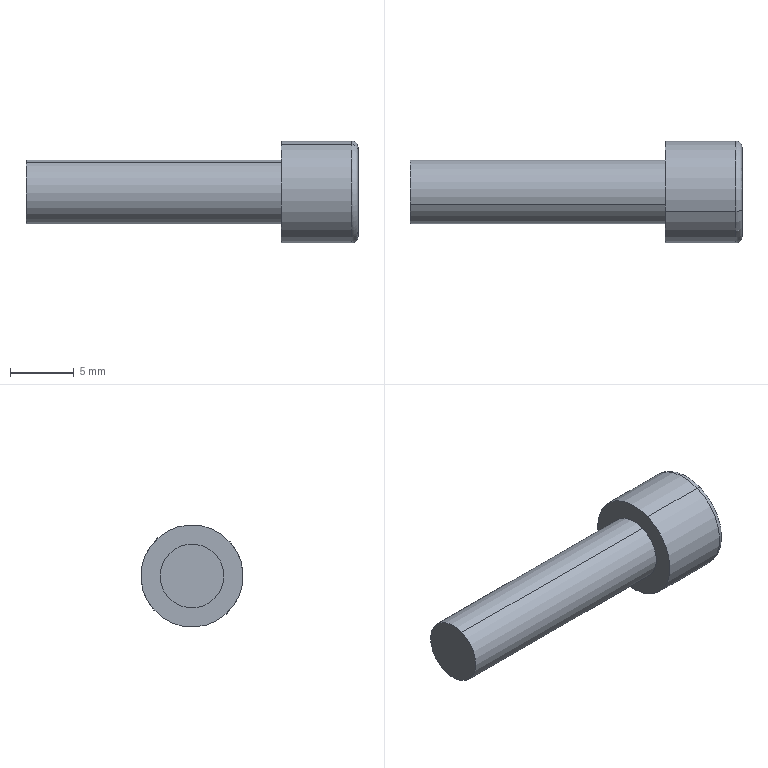Part | SolidWorks | features BaseBody 1 | 1 solid | 16 faces | box 26 x 8 x 8 mm | volume 606.379 mm3 | plane 10 | cylinder 4 | torus 2 | commonest cylinder face diameters 5 x2 8 x2
STEP:
#1=CARTESIAN_POINT('',(373.577,490.167,331.412));
#2=VERTEX_POINT('',#1);
#3=CARTESIAN_POINT('',(374.077,489.976,331.874));
#4=VERTEX_POINT('',#3);
#5=CARTESIAN_POINT('',(373.577,489.976,331.874));
#6=DIRECTION('',(0.,-0.9237,-0.383));
#7=DIRECTION('',(0.,0.383,-0.9237));
#8=AXIS2_PLACEMENT_3D('',#5,#6,#7);
#9=CIRCLE('',#8,0.5);
#10=EDGE_CURVE('',#2,#4,#9,.T.);
#11=ORIENTED_EDGE('',*,*,#10,.T.);
#12=CARTESIAN_POINT('',(374.077,487.294,338.34));
#13=VERTEX_POINT('',#12);
#14=CARTESIAN_POINT('',(374.077,488.635,335.107));
#15=DIRECTION('',(1.,0.,0.));
#16=DIRECTION('',(0.,-0.383,0.9237));
#17=AXIS2_PLACEMENT_3D('',#14,#15,#16);
#18=CIRCLE('',#17,3.5);
#19=EDGE_CURVE('',#13,#4,#18,.T.);
#20=ORIENTED_EDGE('',*,*,#19,.F.);
#21=CARTESIAN_POINT('',(373.577,487.103,338.802));
#22=VERTEX_POINT('',#21);
#23=CARTESIAN_POINT('',(373.577,487.294,338.34));
#24=DIRECTION('',(0.,0.9237,0.383));
#25=DIRECTION('',(1.,0.,0.));
#26=AXIS2_PLACEMENT_3D('',#23,#24,#25);
#27=CIRCLE('',#26,0.5);
#28=EDGE_CURVE('',#22,#13,#27,.T.);
#29=ORIENTED_EDGE('',*,*,#28,.F.);
#30=CARTESIAN_POINT('',(373.577,488.635,335.107));
#31=DIRECTION('',(-1.,0.,0.));
#32=DIRECTION('',(0.,-0.383,0.9237));
#33=AXIS2_PLACEMENT_3D('',#30,#31,#32);
#34=CIRCLE('',#33,4.);
#35=EDGE_CURVE('',#2,#22,#34,.T.);
#36=ORIENTED_EDGE('',*,*,#35,.F.);
#37=EDGE_LOOP('',(#11,#20,#29,#36));
#38=FACE_OUTER_BOUND('',#37,.T.);
#39=CARTESIAN_POINT('',(373.577,488.635,335.107));
#40=DIRECTION('',(-1.,0.,0.));
#41=DIRECTION('',(0.,0.383,-0.9237));
#42=AXIS2_PLACEMENT_3D('',#39,#40,#41);
#43=TOROIDAL_SURFACE('',#42,3.5,0.5);
#44=ADVANCED_FACE('',(#38),#43,.T.);
#45=CARTESIAN_POINT('',(370.077,490.7,333.09));
#46=VERTEX_POINT('',#45);
#47=CARTESIAN_POINT('',(370.077,487.921,332.31));
#48=VERTEX_POINT('',#47);
#49=CARTESIAN_POINT('',(370.077,480.763,330.301));
#50=DIRECTION('',(0.,-0.9628,-0.2702));
#51=VECTOR('',#50,1000.);
#52=LINE('',#49,#51);
#53=EDGE_CURVE('',#46,#48,#52,.T.);
#54=ORIENTED_EDGE('',*,*,#53,.F.);
#55=CARTESIAN_POINT('',(370.077,491.414,335.887));
#56=VERTEX_POINT('',#55);
#57=CARTESIAN_POINT('',(370.077,489.731,329.293));
#58=DIRECTION('',(0.,-0.2474,-0.9689));
#59=VECTOR('',#58,1000.);
#60=LINE('',#57,#59);
#61=EDGE_CURVE('',#56,#46,#60,.T.);
#62=ORIENTED_EDGE('',*,*,#61,.F.);
#63=CARTESIAN_POINT('',(370.077,489.349,337.904));
#64=VERTEX_POINT('',#63);
#65=CARTESIAN_POINT('',(370.077,489.349,337.904));
#66=DIRECTION('',(0.,0.7154,-0.6987));
#67=VECTOR('',#66,1000.);
#68=LINE('',#65,#67);
#69=EDGE_CURVE('',#64,#56,#68,.T.);
#70=ORIENTED_EDGE('',*,*,#69,.F.);
#71=CARTESIAN_POINT('',(370.077,486.57,337.124));
#72=VERTEX_POINT('',#71);
#73=CARTESIAN_POINT('',(370.077,486.57,337.124));
#74=DIRECTION('',(0.,0.9628,0.2702));
#75=VECTOR('',#74,1000.);
#76=LINE('',#73,#75);
#77=EDGE_CURVE('',#72,#64,#76,.T.);
#78=ORIENTED_EDGE('',*,*,#77,.F.);
#79=CARTESIAN_POINT('',(370.077,485.855,334.327));
#80=VERTEX_POINT('',#79);
#81=CARTESIAN_POINT('',(370.077,485.855,334.327));
#82=DIRECTION('',(0.,0.2474,0.9689));
#83=VECTOR('',#82,1000.);
#84=LINE('',#81,#83);
#85=EDGE_CURVE('',#80,#72,#84,.T.);
#86=ORIENTED_EDGE('',*,*,#85,.F.);
#87=CARTESIAN_POINT('',(370.077,487.921,332.31));
#88=DIRECTION('',(0.,-0.7154,0.6987));
#89=VECTOR('',#88,1000.);
#90=LINE('',#87,#89);
#91=EDGE_CURVE('',#48,#80,#90,.T.);
#92=ORIENTED_EDGE('',*,*,#91,.F.);
#93=EDGE_LOOP('',(#54,#62,#70,#78,#86,#92));
#94=FACE_OUTER_BOUND('',#93,.T.);
#95=CARTESIAN_POINT('',(370.077,480.375,331.682));
#96=DIRECTION('',(-1.,0.,0.));
#97=DIRECTION('',(0.,0.,1.));
#98=AXIS2_PLACEMENT_3D('',#95,#96,#97);
#99=PLANE('',#98);
#100=ADVANCED_FACE('',(#94),#99,.F.);
#101=CARTESIAN_POINT('',(374.077,487.921,332.31));
#102=VERTEX_POINT('',#101);
#103=CARTESIAN_POINT('',(390.077,487.921,332.31));
#104=DIRECTION('',(-1.,0.,0.));
#105=VECTOR('',#104,1000.);
#106=LINE('',#103,#105);
#107=EDGE_CURVE('',#102,#48,#106,.T.);
#108=ORIENTED_EDGE('',*,*,#107,.T.);
#109=ORIENTED_EDGE('',*,*,#91,.T.);
#110=CARTESIAN_POINT('',(374.077,485.855,334.327));
#111=VERTEX_POINT('',#110);
#112=CARTESIAN_POINT('',(390.077,485.855,334.327));
#113=DIRECTION('',(-1.,0.,0.));
#114=VECTOR('',#113,1000.);
#115=LINE('',#112,#114);
#116=EDGE_CURVE('',#111,#80,#115,.T.);
#117=ORIENTED_EDGE('',*,*,#116,.F.);
#118=CARTESIAN_POINT('',(374.077,484.373,335.775));
#119=DIRECTION('',(0.,-0.7154,0.6987));
#120=VECTOR('',#119,1000.);
#121=LINE('',#118,#120);
#122=EDGE_CURVE('',#102,#111,#121,.T.);
#123=ORIENTED_EDGE('',*,*,#122,.F.);
#124=EDGE_LOOP('',(#108,#109,#117,#123));
#125=FACE_OUTER_BOUND('',#124,.T.);
#126=CARTESIAN_POINT('',(390.077,487.921,332.31));
#127=DIRECTION('',(0.,-0.6987,-0.7154));
#128=DIRECTION('',(0.,-0.7154,0.6987));
#129=AXIS2_PLACEMENT_3D('',#126,#127,#128);
#130=PLANE('',#129);
#131=ADVANCED_FACE('',(#125),#130,.F.);
#132=ORIENTED_EDGE('',*,*,#116,.T.);
#133=ORIENTED_EDGE('',*,*,#85,.T.);
#134=CARTESIAN_POINT('',(374.077,486.57,337.124));
#135=VERTEX_POINT('',#134);
#136=CARTESIAN_POINT('',(390.077,486.57,337.124));
#137=DIRECTION('',(-1.,0.,0.));
#138=VECTOR('',#137,1000.);
#139=LINE('',#136,#138);
#140=EDGE_CURVE('',#135,#72,#139,.T.);
#141=ORIENTED_EDGE('',*,*,#140,.F.);
#142=CARTESIAN_POINT('',(374.077,484.886,330.53));
#143=DIRECTION('',(0.,0.2474,0.9689));
#144=VECTOR('',#143,1000.);
#145=LINE('',#142,#144);
#146=EDGE_CURVE('',#111,#135,#145,.T.);
#147=ORIENTED_EDGE('',*,*,#146,.F.);
#148=EDGE_LOOP('',(#132,#133,#141,#147));
#149=FACE_OUTER_BOUND('',#148,.T.);
#150=CARTESIAN_POINT('',(390.077,485.855,334.327));
#151=DIRECTION('',(0.,-0.9689,0.2474));
#152=DIRECTION('',(-1.,0.,0.));
#153=AXIS2_PLACEMENT_3D('',#150,#151,#152);
#154=PLANE('',#153);
#155=ADVANCED_FACE('',(#149),#154,.F.);
#156=ORIENTED_EDGE('',*,*,#140,.T.);
#157=ORIENTED_EDGE('',*,*,#77,.T.);
#158=CARTESIAN_POINT('',(374.077,489.349,337.904));
#159=VERTEX_POINT('',#158);
#160=CARTESIAN_POINT('',(390.077,489.349,337.904));
#161=DIRECTION('',(-1.,0.,0.));
#162=VECTOR('',#161,1000.);
#163=LINE('',#160,#162);
#164=EDGE_CURVE('',#159,#64,#163,.T.);
#165=ORIENTED_EDGE('',*,*,#164,.F.);
#166=CARTESIAN_POINT('',(374.077,479.412,335.115));
#167=DIRECTION('',(0.,0.9628,0.2702));
#168=VECTOR('',#167,1000.);
#169=LINE('',#166,#168);
#170=EDGE_CURVE('',#135,#159,#169,.T.);
#171=ORIENTED_EDGE('',*,*,#170,.F.);
#172=EDGE_LOOP('',(#156,#157,#165,#171));
#173=FACE_OUTER_BOUND('',#172,.T.);
#174=CARTESIAN_POINT('',(390.077,486.57,337.124));
#175=DIRECTION('',(0.,-0.2702,0.9628));
#176=DIRECTION('',(-1.,0.,0.));
#177=AXIS2_PLACEMENT_3D('',#174,#175,#176);
#178=PLANE('',#177);
#179=ADVANCED_FACE('',(#173),#178,.F.);
#180=ORIENTED_EDGE('',*,*,#164,.T.);
#181=ORIENTED_EDGE('',*,*,#69,.T.);
#182=CARTESIAN_POINT('',(374.077,491.414,335.887));
#183=VERTEX_POINT('',#182);
#184=CARTESIAN_POINT('',(390.077,491.414,335.887));
#185=DIRECTION('',(-1.,0.,0.));
#186=VECTOR('',#185,1000.);
#187=LINE('',#184,#186);
#188=EDGE_CURVE('',#183,#56,#187,.T.);
#189=ORIENTED_EDGE('',*,*,#188,.F.);
#190=CARTESIAN_POINT('',(374.077,487.866,339.352));
#191=DIRECTION('',(0.,0.7154,-0.6987));
#192=VECTOR('',#191,1000.);
#193=LINE('',#190,#192);
#194=EDGE_CURVE('',#159,#183,#193,.T.);
#195=ORIENTED_EDGE('',*,*,#194,.F.);
#196=EDGE_LOOP('',(#180,#181,#189,#195));
#197=FACE_OUTER_BOUND('',#196,.T.);
#198=CARTESIAN_POINT('',(390.077,489.349,337.904));
#199=DIRECTION('',(0.,0.6987,0.7154));
#200=DIRECTION('',(1.,0.,0.));
#201=AXIS2_PLACEMENT_3D('',#198,#199,#200);
#202=PLANE('',#201);
#203=ADVANCED_FACE('',(#197),#202,.F.);
#204=ORIENTED_EDGE('',*,*,#188,.T.);
#205=ORIENTED_EDGE('',*,*,#61,.T.);
#206=CARTESIAN_POINT('',(374.077,490.7,333.09));
#207=VERTEX_POINT('',#206);
#208=CARTESIAN_POINT('',(390.077,490.7,333.09));
#209=DIRECTION('',(-1.,0.,0.));
#210=VECTOR('',#209,1000.);
#211=LINE('',#208,#210);
#212=EDGE_CURVE('',#207,#46,#211,.T.);
#213=ORIENTED_EDGE('',*,*,#212,.F.);
#214=CARTESIAN_POINT('',(374.077,489.731,329.293));
#215=DIRECTION('',(0.,-0.2474,-0.9689));
#216=VECTOR('',#215,1000.);
#217=LINE('',#214,#216);
#218=EDGE_CURVE('',#183,#207,#217,.T.);
#219=ORIENTED_EDGE('',*,*,#218,.F.);
#220=EDGE_LOOP('',(#204,#205,#213,#219));
#221=FACE_OUTER_BOUND('',#220,.T.);
#222=CARTESIAN_POINT('',(390.077,489.731,329.293));
#223=DIRECTION('',(0.,0.9689,-0.2474));
#224=DIRECTION('',(-1.,0.,0.));
#225=AXIS2_PLACEMENT_3D('',#222,#223,#224);
#226=PLANE('',#225);
#227=ADVANCED_FACE('',(#221),#226,.F.);
#228=ORIENTED_EDGE('',*,*,#212,.T.);
#229=ORIENTED_EDGE('',*,*,#53,.T.);
#230=ORIENTED_EDGE('',*,*,#107,.F.);
#231=CARTESIAN_POINT('',(374.077,480.763,330.301));
#232=DIRECTION('',(0.,-0.9628,-0.2702));
#233=VECTOR('',#232,1000.);
#234=LINE('',#231,#233);
#235=EDGE_CURVE('',#207,#102,#234,.T.);
#236=ORIENTED_EDGE('',*,*,#235,.F.);
#237=EDGE_LOOP('',(#228,#229,#230,#236));
#238=FACE_OUTER_BOUND('',#237,.T.);
#239=CARTESIAN_POINT('',(390.077,480.763,330.301));
#240=DIRECTION('',(0.,0.2702,-0.9628));
#241=DIRECTION('',(-1.,0.,0.));
#242=AXIS2_PLACEMENT_3D('',#239,#240,#241);
#243=PLANE('',#242);
#244=ADVANCED_FACE('',(#238),#243,.F.);
#245=ORIENTED_EDGE('',*,*,#218,.T.);
#246=ORIENTED_EDGE('',*,*,#235,.T.);
#247=ORIENTED_EDGE('',*,*,#122,.T.);
#248=ORIENTED_EDGE('',*,*,#146,.T.);
#249=ORIENTED_EDGE('',*,*,#170,.T.);
#250=ORIENTED_EDGE('',*,*,#194,.T.);
#251=EDGE_LOOP('',(#245,#246,#247,#248,#249,#250));
#252=FACE_BOUND('',#251,.T.);
#253=ORIENTED_EDGE('',*,*,#19,.T.);
#254=CARTESIAN_POINT('',(374.077,488.635,335.107));
#255=DIRECTION('',(1.,0.,0.));
#256=DIRECTION('',(0.,-0.383,0.9237));
#257=AXIS2_PLACEMENT_3D('',#254,#255,#256);
#258=CIRCLE('',#257,3.5);
#259=EDGE_CURVE('',#4,#13,#258,.T.);
#260=ORIENTED_EDGE('',*,*,#259,.T.);
#261=EDGE_LOOP('',(#253,#260));
#262=FACE_OUTER_BOUND('',#261,.T.);
#263=CARTESIAN_POINT('',(374.077,480.375,331.682));
#264=DIRECTION('',(-1.,0.,0.));
#265=DIRECTION('',(0.,0.,1.));
#266=AXIS2_PLACEMENT_3D('',#263,#264,#265);
#267=PLANE('',#266);
#268=ADVANCED_FACE('',(#252,#262),#267,.F.);
#269=CARTESIAN_POINT('',(368.077,490.167,331.412));
#270=VERTEX_POINT('',#269);
#271=CARTESIAN_POINT('',(374.077,490.167,331.412));
#272=DIRECTION('',(1.,0.,0.));
#273=VECTOR('',#272,1000.);
#274=LINE('',#271,#273);
#275=EDGE_CURVE('',#270,#2,#274,.T.);
#276=ORIENTED_EDGE('',*,*,#275,.T.);
#277=ORIENTED_EDGE('',*,*,#35,.T.);
#278=CARTESIAN_POINT('',(368.077,487.103,338.802));
#279=VERTEX_POINT('',#278);
#280=CARTESIAN_POINT('',(374.077,487.103,338.802));
#281=DIRECTION('',(1.,0.,0.));
#282=VECTOR('',#281,1000.);
#283=LINE('',#280,#282);
#284=EDGE_CURVE('',#279,#22,#283,.T.);
#285=ORIENTED_EDGE('',*,*,#284,.F.);
#286=CARTESIAN_POINT('',(368.077,488.635,335.107));
#287=DIRECTION('',(-1.,0.,0.));
#288=DIRECTION('',(0.,-0.383,0.9237));
#289=AXIS2_PLACEMENT_3D('',#286,#287,#288);
#290=CIRCLE('',#289,4.);
#291=EDGE_CURVE('',#270,#279,#290,.T.);
#292=ORIENTED_EDGE('',*,*,#291,.F.);
#293=EDGE_LOOP('',(#276,#277,#285,#292));
#294=FACE_OUTER_BOUND('',#293,.T.);
#295=CARTESIAN_POINT('',(374.077,488.635,335.107));
#296=DIRECTION('',(-1.,0.,0.));
#297=DIRECTION('',(0.,0.383,-0.9237));
#298=AXIS2_PLACEMENT_3D('',#295,#296,#297);
#299=CYLINDRICAL_SURFACE('',#298,4.);
#300=ADVANCED_FACE('',(#294),#299,.T.);
#301=CARTESIAN_POINT('',(368.077,489.592,332.797));
#302=VERTEX_POINT('',#301);
#303=CARTESIAN_POINT('',(368.077,487.677,337.416));
#304=VERTEX_POINT('',#303);
#305=CARTESIAN_POINT('',(368.077,488.635,335.107));
#306=DIRECTION('',(-1.,0.,0.));
#307=DIRECTION('',(0.,-0.383,0.9237));
#308=AXIS2_PLACEMENT_3D('',#305,#306,#307);
#309=CIRCLE('',#308,2.5);
#310=EDGE_CURVE('',#302,#304,#309,.T.);
#311=ORIENTED_EDGE('',*,*,#310,.F.);
#312=CARTESIAN_POINT('',(368.077,488.635,335.107));
#313=DIRECTION('',(-1.,0.,0.));
#314=DIRECTION('',(0.,-0.383,0.9237));
#315=AXIS2_PLACEMENT_3D('',#312,#313,#314);
#316=CIRCLE('',#315,2.5);
#317=EDGE_CURVE('',#304,#302,#316,.T.);
#318=ORIENTED_EDGE('',*,*,#317,.F.);
#319=EDGE_LOOP('',(#311,#318));
#320=FACE_BOUND('',#319,.T.);
#321=CARTESIAN_POINT('',(368.077,488.635,335.107));
#322=DIRECTION('',(-1.,0.,0.));
#323=DIRECTION('',(0.,-0.383,0.9237));
#324=AXIS2_PLACEMENT_3D('',#321,#322,#323);
#325=CIRCLE('',#324,4.);
#326=EDGE_CURVE('',#279,#270,#325,.T.);
#327=ORIENTED_EDGE('',*,*,#326,.T.);
#328=ORIENTED_EDGE('',*,*,#291,.T.);
#329=EDGE_LOOP('',(#327,#328));
#330=FACE_OUTER_BOUND('',#329,.T.);
#331=CARTESIAN_POINT('',(368.077,480.375,331.682));
#332=DIRECTION('',(-1.,0.,0.));
#333=DIRECTION('',(0.,0.,1.));
#334=AXIS2_PLACEMENT_3D('',#331,#332,#333);
#335=PLANE('',#334);
#336=ADVANCED_FACE('',(#320,#330),#335,.T.);
#337=CARTESIAN_POINT('',(348.077,489.592,332.797));
#338=VERTEX_POINT('',#337);
#339=CARTESIAN_POINT('',(348.077,487.677,337.416));
#340=VERTEX_POINT('',#339);
#341=CARTESIAN_POINT('',(348.077,488.635,335.107));
#342=DIRECTION('',(-1.,0.,0.));
#343=DIRECTION('',(0.,-0.383,0.9237));
#344=AXIS2_PLACEMENT_3D('',#341,#342,#343);
#345=CIRCLE('',#344,2.5);
#346=EDGE_CURVE('',#338,#340,#345,.T.);
#347=ORIENTED_EDGE('',*,*,#346,.T.);
#348=CARTESIAN_POINT('',(348.077,488.635,335.107));
#349=DIRECTION('',(-1.,0.,0.));
#350=DIRECTION('',(0.,-0.383,0.9237));
#351=AXIS2_PLACEMENT_3D('',#348,#349,#350);
#352=CIRCLE('',#351,2.5);
#353=EDGE_CURVE('',#340,#338,#352,.T.);
#354=ORIENTED_EDGE('',*,*,#353,.T.);
#355=EDGE_LOOP('',(#347,#354));
#356=FACE_OUTER_BOUND('',#355,.T.);
#357=CARTESIAN_POINT('',(348.077,480.375,331.682));
#358=DIRECTION('',(-1.,0.,0.));
#359=DIRECTION('',(0.,0.,1.));
#360=AXIS2_PLACEMENT_3D('',#357,#358,#359);
#361=PLANE('',#360);
#362=ADVANCED_FACE('',(#356),#361,.T.);
#363=CARTESIAN_POINT('',(348.077,487.677,337.416));
#364=DIRECTION('',(-1.,0.,0.));
#365=VECTOR('',#364,1000.);
#366=LINE('',#363,#365);
#367=EDGE_CURVE('',#304,#340,#366,.T.);
#368=ORIENTED_EDGE('',*,*,#367,.T.);
#369=ORIENTED_EDGE('',*,*,#346,.F.);
#370=CARTESIAN_POINT('',(348.077,489.592,332.797));
#371=DIRECTION('',(-1.,0.,0.));
#372=VECTOR('',#371,1000.);
#373=LINE('',#370,#372);
#374=EDGE_CURVE('',#302,#338,#373,.T.);
#375=ORIENTED_EDGE('',*,*,#374,.F.);
#376=ORIENTED_EDGE('',*,*,#310,.T.);
#377=EDGE_LOOP('',(#368,#369,#375,#376));
#378=FACE_OUTER_BOUND('',#377,.T.);
#379=CARTESIAN_POINT('',(348.077,488.635,335.107));
#380=DIRECTION('',(1.,0.,0.));
#381=DIRECTION('',(0.,-0.383,0.9237));
#382=AXIS2_PLACEMENT_3D('',#379,#380,#381);
#383=CYLINDRICAL_SURFACE('',#382,2.5);
#384=ADVANCED_FACE('',(#378),#383,.T.);
#385=ORIENTED_EDGE('',*,*,#353,.F.);
#386=ORIENTED_EDGE('',*,*,#367,.F.);
#387=ORIENTED_EDGE('',*,*,#317,.T.);
#388=ORIENTED_EDGE('',*,*,#374,.T.);
#389=EDGE_LOOP('',(#385,#386,#387,#388));
#390=FACE_OUTER_BOUND('',#389,.T.);
#391=CARTESIAN_POINT('',(348.077,488.635,335.107));
#392=DIRECTION('',(1.,0.,0.));
#393=DIRECTION('',(0.,-0.383,0.9237));
#394=AXIS2_PLACEMENT_3D('',#391,#392,#393);
#395=CYLINDRICAL_SURFACE('',#394,2.5);
#396=ADVANCED_FACE('',(#390),#395,.T.);
#397=CARTESIAN_POINT('',(373.577,488.635,335.107));
#398=DIRECTION('',(-1.,0.,0.));
#399=DIRECTION('',(0.,-0.383,0.9237));
#400=AXIS2_PLACEMENT_3D('',#397,#398,#399);
#401=CIRCLE('',#400,4.);
#402=EDGE_CURVE('',#22,#2,#401,.T.);
#403=ORIENTED_EDGE('',*,*,#402,.T.);
#404=ORIENTED_EDGE('',*,*,#275,.F.);
#405=ORIENTED_EDGE('',*,*,#326,.F.);
#406=ORIENTED_EDGE('',*,*,#284,.T.);
#407=EDGE_LOOP('',(#403,#404,#405,#406));
#408=FACE_OUTER_BOUND('',#407,.T.);
#409=CARTESIAN_POINT('',(374.077,488.635,335.107));
#410=DIRECTION('',(-1.,0.,0.));
#411=DIRECTION('',(0.,0.383,-0.9237));
#412=AXIS2_PLACEMENT_3D('',#409,#410,#411);
#413=CYLINDRICAL_SURFACE('',#412,4.);
#414=ADVANCED_FACE('',(#408),#413,.T.);
#415=ORIENTED_EDGE('',*,*,#259,.F.);
#416=ORIENTED_EDGE('',*,*,#10,.F.);
#417=ORIENTED_EDGE('',*,*,#402,.F.);
#418=ORIENTED_EDGE('',*,*,#28,.T.);
#419=EDGE_LOOP('',(#415,#416,#417,#418));
#420=FACE_OUTER_BOUND('',#419,.T.);
#421=CARTESIAN_POINT('',(373.577,488.635,335.107));
#422=DIRECTION('',(-1.,0.,0.));
#423=DIRECTION('',(0.,0.383,-0.9237));
#424=AXIS2_PLACEMENT_3D('',#421,#422,#423);
#425=TOROIDAL_SURFACE('',#424,3.5,0.5);
#426=ADVANCED_FACE('',(#420),#425,.T.);
#427=CLOSED_SHELL('',(#44,#100,#131,#155,#179,#203,#227,#244,#268,#300,#336,#362,#384,#396,#414,#426));
#428=MANIFOLD_SOLID_BREP('',#427);
#429=CARTESIAN_POINT('',(0.,0.,0.));
#430=DIRECTION('',(0.,0.,1.));
#431=DIRECTION('',(1.,0.,0.));
#432=AXIS2_PLACEMENT_3D('',#429,#430,#431);
#433=(LENGTH_UNIT()NAMED_UNIT(*)SI_UNIT(.MILLI.,.METRE.));
#434=UNCERTAINTY_MEASURE_WITH_UNIT(LENGTH_MEASURE(0.00001),#433,'','');
#435=(NAMED_UNIT(*)PLANE_ANGLE_UNIT()SI_UNIT($,.RADIAN.));
#436=(NAMED_UNIT(*)SI_UNIT($,.STERADIAN.)SOLID_ANGLE_UNIT());
#437=(GEOMETRIC_REPRESENTATION_CONTEXT(3)GLOBAL_UNCERTAINTY_ASSIGNED_CONTEXT((#434))GLOBAL_UNIT_ASSIGNED_CONTEXT((#433,#435,#436))REPRESENTATION_CONTEXT('',''));
#438=ADVANCED_BREP_SHAPE_REPRESENTATION('',(#428,#432),#437);